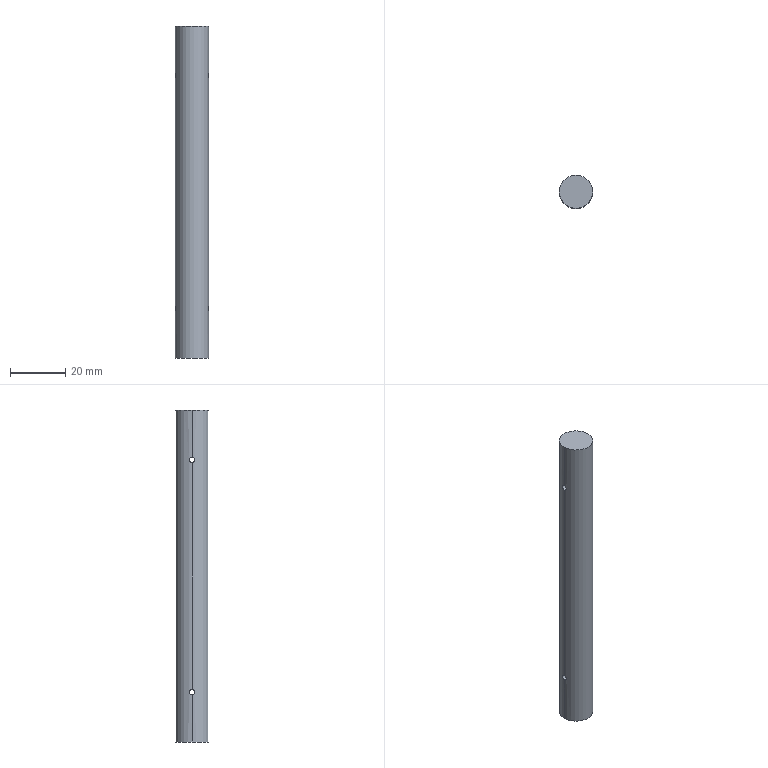Part | SolidWorks | features Cut 1, Extrusion 1 | 1 solid | 8 faces | box 12 x 12 x 120 mm | volume 13497 mm3 | cylinder 6 | plane 2 | commonest cylinder face diameters 2 x4 12 x2
STEP:
#1=CARTESIAN_POINT('',(-94.,71.3,-41.));
#2=VERTEX_POINT('',#1);
#3=CARTESIAN_POINT('',(-94.,71.3,-43.));
#4=VERTEX_POINT('',#3);
#5=CARTESIAN_POINT('',(-94.,71.3,-41.));
#6=CARTESIAN_POINT('',(-94.,71.168,-41.));
#7=CARTESIAN_POINT('',(-94.005,71.038,-41.026));
#8=CARTESIAN_POINT('',(-94.02,70.796,-41.127));
#9=CARTESIAN_POINT('',(-94.031,70.685,-41.201));
#10=CARTESIAN_POINT('',(-94.053,70.501,-41.385));
#11=CARTESIAN_POINT('',(-94.064,70.426,-41.497));
#12=CARTESIAN_POINT('',(-94.079,70.326,-41.737));
#13=CARTESIAN_POINT('',(-94.084,70.3,-41.869));
#14=CARTESIAN_POINT('',(-94.084,70.3,-42.13));
#15=CARTESIAN_POINT('',(-94.079,70.326,-42.261));
#16=CARTESIAN_POINT('',(-94.064,70.426,-42.504));
#17=CARTESIAN_POINT('',(-94.053,70.5,-42.614));
#18=CARTESIAN_POINT('',(-94.031,70.686,-42.8));
#19=CARTESIAN_POINT('',(-94.02,70.796,-42.874));
#20=CARTESIAN_POINT('',(-94.004,71.038,-42.974));
#21=CARTESIAN_POINT('',(-94.,71.169,-43.));
#22=CARTESIAN_POINT('',(-94.,71.3,-43.));
#23=B_SPLINE_CURVE_WITH_KNOTS('',3,(#5,#6,#7,#8,#9,#10,#11,#12,#13,#14,#15,#16,#17,#18,#19,#20,#21,#22),.UNSPECIFIED.,.F.,.F.,(4,2,2,2,2,2,2,2,4),(0.,0.0003915,0.000783,0.001174,0.001566,0.001957,0.002349,0.00274,0.003132),.UNSPECIFIED.);
#24=EDGE_CURVE('',#2,#4,#23,.T.);
#25=ORIENTED_EDGE('',*,*,#24,.T.);
#26=CARTESIAN_POINT('',(-106.,71.3,-43.));
#27=VERTEX_POINT('',#26);
#28=CARTESIAN_POINT('',(-94.,71.3,-43.));
#29=DIRECTION('',(-1.,0.,0.));
#30=VECTOR('',#29,1000.);
#31=LINE('',#28,#30);
#32=EDGE_CURVE('',#4,#27,#31,.T.);
#33=ORIENTED_EDGE('',*,*,#32,.T.);
#34=CARTESIAN_POINT('',(-106.,71.3,-41.));
#35=VERTEX_POINT('',#34);
#36=CARTESIAN_POINT('',(-106.,71.3,-43.));
#37=CARTESIAN_POINT('',(-106.,71.169,-43.));
#38=CARTESIAN_POINT('',(-105.995,71.038,-42.974));
#39=CARTESIAN_POINT('',(-105.98,70.797,-42.874));
#40=CARTESIAN_POINT('',(-105.969,70.686,-42.8));
#41=CARTESIAN_POINT('',(-105.947,70.501,-42.615));
#42=CARTESIAN_POINT('',(-105.936,70.427,-42.505));
#43=CARTESIAN_POINT('',(-105.921,70.326,-42.263));
#44=CARTESIAN_POINT('',(-105.916,70.3,-42.133));
#45=CARTESIAN_POINT('',(-105.916,70.3,-41.868));
#46=CARTESIAN_POINT('',(-105.921,70.326,-41.738));
#47=CARTESIAN_POINT('',(-105.936,70.426,-41.496));
#48=CARTESIAN_POINT('',(-105.947,70.5,-41.385));
#49=CARTESIAN_POINT('',(-105.969,70.684,-41.201));
#50=CARTESIAN_POINT('',(-105.98,70.796,-41.127));
#51=CARTESIAN_POINT('',(-105.995,71.036,-41.027));
#52=CARTESIAN_POINT('',(-106.,71.168,-41.));
#53=CARTESIAN_POINT('',(-106.,71.3,-41.));
#54=B_SPLINE_CURVE_WITH_KNOTS('',3,(#36,#37,#38,#39,#40,#41,#42,#43,#44,#45,#46,#47,#48,#49,#50,#51,#52,#53),.UNSPECIFIED.,.F.,.F.,(4,2,2,2,2,2,2,2,4),(0.003132,0.003523,0.003915,0.004306,0.004697,0.005089,0.00548,0.005872,0.006263),.UNSPECIFIED.);
#55=EDGE_CURVE('',#27,#35,#54,.T.);
#56=ORIENTED_EDGE('',*,*,#55,.T.);
#57=CARTESIAN_POINT('',(-94.,71.3,-41.));
#58=DIRECTION('',(-1.,0.,0.));
#59=VECTOR('',#58,1000.);
#60=LINE('',#57,#59);
#61=EDGE_CURVE('',#2,#35,#60,.T.);
#62=ORIENTED_EDGE('',*,*,#61,.F.);
#63=EDGE_LOOP('',(#25,#33,#56,#62));
#64=FACE_OUTER_BOUND('',#63,.T.);
#65=CARTESIAN_POINT('',(-94.,71.3,-42.));
#66=DIRECTION('',(-1.,0.,0.));
#67=DIRECTION('',(0.,0.,1.));
#68=AXIS2_PLACEMENT_3D('',#65,#66,#67);
#69=CYLINDRICAL_SURFACE('',#68,1.);
#70=ADVANCED_FACE('',(#64),#69,.F.);
#71=CARTESIAN_POINT('',(-94.,71.3,43.));
#72=VERTEX_POINT('',#71);
#73=CARTESIAN_POINT('',(-94.,71.3,41.));
#74=VERTEX_POINT('',#73);
#75=CARTESIAN_POINT('',(-94.,71.3,43.));
#76=CARTESIAN_POINT('',(-94.,71.168,43.));
#77=CARTESIAN_POINT('',(-94.005,71.038,42.974));
#78=CARTESIAN_POINT('',(-94.02,70.796,42.873));
#79=CARTESIAN_POINT('',(-94.031,70.685,42.799));
#80=CARTESIAN_POINT('',(-94.053,70.501,42.615));
#81=CARTESIAN_POINT('',(-94.064,70.426,42.503));
#82=CARTESIAN_POINT('',(-94.079,70.326,42.263));
#83=CARTESIAN_POINT('',(-94.084,70.3,42.131));
#84=CARTESIAN_POINT('',(-94.084,70.3,41.87));
#85=CARTESIAN_POINT('',(-94.079,70.326,41.739));
#86=CARTESIAN_POINT('',(-94.064,70.426,41.496));
#87=CARTESIAN_POINT('',(-94.053,70.5,41.386));
#88=CARTESIAN_POINT('',(-94.031,70.686,41.2));
#89=CARTESIAN_POINT('',(-94.02,70.796,41.126));
#90=CARTESIAN_POINT('',(-94.004,71.038,41.026));
#91=CARTESIAN_POINT('',(-94.,71.169,41.));
#92=CARTESIAN_POINT('',(-94.,71.3,41.));
#93=B_SPLINE_CURVE_WITH_KNOTS('',3,(#75,#76,#77,#78,#79,#80,#81,#82,#83,#84,#85,#86,#87,#88,#89,#90,#91,#92),.UNSPECIFIED.,.F.,.F.,(4,2,2,2,2,2,2,2,4),(0.,0.0003915,0.000783,0.001174,0.001566,0.001957,0.002349,0.00274,0.003132),.UNSPECIFIED.);
#94=EDGE_CURVE('',#72,#74,#93,.T.);
#95=ORIENTED_EDGE('',*,*,#94,.T.);
#96=CARTESIAN_POINT('',(-106.,71.3,41.));
#97=VERTEX_POINT('',#96);
#98=CARTESIAN_POINT('',(-94.,71.3,41.));
#99=DIRECTION('',(-1.,0.,0.));
#100=VECTOR('',#99,1000.);
#101=LINE('',#98,#100);
#102=EDGE_CURVE('',#74,#97,#101,.T.);
#103=ORIENTED_EDGE('',*,*,#102,.T.);
#104=CARTESIAN_POINT('',(-106.,71.3,43.));
#105=VERTEX_POINT('',#104);
#106=CARTESIAN_POINT('',(-106.,71.3,41.));
#107=CARTESIAN_POINT('',(-106.,71.169,41.));
#108=CARTESIAN_POINT('',(-105.995,71.038,41.026));
#109=CARTESIAN_POINT('',(-105.98,70.797,41.126));
#110=CARTESIAN_POINT('',(-105.969,70.686,41.2));
#111=CARTESIAN_POINT('',(-105.947,70.501,41.385));
#112=CARTESIAN_POINT('',(-105.936,70.427,41.495));
#113=CARTESIAN_POINT('',(-105.921,70.326,41.737));
#114=CARTESIAN_POINT('',(-105.916,70.3,41.867));
#115=CARTESIAN_POINT('',(-105.916,70.3,42.132));
#116=CARTESIAN_POINT('',(-105.921,70.326,42.262));
#117=CARTESIAN_POINT('',(-105.936,70.426,42.504));
#118=CARTESIAN_POINT('',(-105.947,70.5,42.615));
#119=CARTESIAN_POINT('',(-105.969,70.684,42.799));
#120=CARTESIAN_POINT('',(-105.98,70.796,42.873));
#121=CARTESIAN_POINT('',(-105.995,71.036,42.973));
#122=CARTESIAN_POINT('',(-106.,71.168,43.));
#123=CARTESIAN_POINT('',(-106.,71.3,43.));
#124=B_SPLINE_CURVE_WITH_KNOTS('',3,(#106,#107,#108,#109,#110,#111,#112,#113,#114,#115,#116,#117,#118,#119,#120,#121,#122,#123),.UNSPECIFIED.,.F.,.F.,(4,2,2,2,2,2,2,2,4),(0.003132,0.003523,0.003915,0.004306,0.004697,0.005089,0.00548,0.005872,0.006263),.UNSPECIFIED.);
#125=EDGE_CURVE('',#97,#105,#124,.T.);
#126=ORIENTED_EDGE('',*,*,#125,.T.);
#127=CARTESIAN_POINT('',(-94.,71.3,43.));
#128=DIRECTION('',(-1.,0.,0.));
#129=VECTOR('',#128,1000.);
#130=LINE('',#127,#129);
#131=EDGE_CURVE('',#72,#105,#130,.T.);
#132=ORIENTED_EDGE('',*,*,#131,.F.);
#133=EDGE_LOOP('',(#95,#103,#126,#132));
#134=FACE_OUTER_BOUND('',#133,.T.);
#135=CARTESIAN_POINT('',(-94.,71.3,42.));
#136=DIRECTION('',(-1.,0.,0.));
#137=DIRECTION('',(0.,0.,1.));
#138=AXIS2_PLACEMENT_3D('',#135,#136,#137);
#139=CYLINDRICAL_SURFACE('',#138,1.);
#140=ADVANCED_FACE('',(#134),#139,.F.);
#141=CARTESIAN_POINT('',(-106.,71.3,-60.));
#142=VERTEX_POINT('',#141);
#143=CARTESIAN_POINT('',(-94.,71.3,-60.));
#144=VERTEX_POINT('',#143);
#145=CARTESIAN_POINT('',(-100.,71.3,-60.));
#146=DIRECTION('',(0.,0.,-1.));
#147=DIRECTION('',(1.,0.,0.));
#148=AXIS2_PLACEMENT_3D('',#145,#146,#147);
#149=CIRCLE('',#148,6.);
#150=EDGE_CURVE('',#142,#144,#149,.T.);
#151=ORIENTED_EDGE('',*,*,#150,.F.);
#152=CARTESIAN_POINT('',(-106.,71.3,-76.971));
#153=DIRECTION('',(0.,0.,1.));
#154=VECTOR('',#153,1000.);
#155=LINE('',#152,#154);
#156=EDGE_CURVE('',#142,#27,#155,.T.);
#157=ORIENTED_EDGE('',*,*,#156,.T.);
#158=CARTESIAN_POINT('',(-106.,71.3,-41.));
#159=CARTESIAN_POINT('',(-106.,71.432,-41.));
#160=CARTESIAN_POINT('',(-105.995,71.562,-41.026));
#161=CARTESIAN_POINT('',(-105.98,71.804,-41.127));
#162=CARTESIAN_POINT('',(-105.969,71.915,-41.201));
#163=CARTESIAN_POINT('',(-105.947,72.099,-41.385));
#164=CARTESIAN_POINT('',(-105.936,72.174,-41.497));
#165=CARTESIAN_POINT('',(-105.921,72.274,-41.737));
#166=CARTESIAN_POINT('',(-105.916,72.3,-41.869));
#167=CARTESIAN_POINT('',(-105.916,72.3,-42.13));
#168=CARTESIAN_POINT('',(-105.921,72.274,-42.261));
#169=CARTESIAN_POINT('',(-105.936,72.174,-42.504));
#170=CARTESIAN_POINT('',(-105.947,72.1,-42.614));
#171=CARTESIAN_POINT('',(-105.969,71.914,-42.8));
#172=CARTESIAN_POINT('',(-105.98,71.804,-42.874));
#173=CARTESIAN_POINT('',(-105.996,71.562,-42.974));
#174=CARTESIAN_POINT('',(-106.,71.431,-43.));
#175=CARTESIAN_POINT('',(-106.,71.3,-43.));
#176=B_SPLINE_CURVE_WITH_KNOTS('',3,(#158,#159,#160,#161,#162,#163,#164,#165,#166,#167,#168,#169,#170,#171,#172,#173,#174,#175),.UNSPECIFIED.,.F.,.F.,(4,2,2,2,2,2,2,2,4),(0.,0.0003915,0.000783,0.001174,0.001566,0.001957,0.002349,0.00274,0.003132),.UNSPECIFIED.);
#177=EDGE_CURVE('',#35,#27,#176,.T.);
#178=ORIENTED_EDGE('',*,*,#177,.F.);
#179=CARTESIAN_POINT('',(-106.,71.3,-76.971));
#180=DIRECTION('',(0.,0.,1.));
#181=VECTOR('',#180,1000.);
#182=LINE('',#179,#181);
#183=EDGE_CURVE('',#35,#97,#182,.T.);
#184=ORIENTED_EDGE('',*,*,#183,.T.);
#185=CARTESIAN_POINT('',(-106.,71.3,43.));
#186=CARTESIAN_POINT('',(-106.,71.432,43.));
#187=CARTESIAN_POINT('',(-105.995,71.562,42.974));
#188=CARTESIAN_POINT('',(-105.98,71.804,42.873));
#189=CARTESIAN_POINT('',(-105.969,71.915,42.799));
#190=CARTESIAN_POINT('',(-105.947,72.099,42.615));
#191=CARTESIAN_POINT('',(-105.936,72.174,42.503));
#192=CARTESIAN_POINT('',(-105.921,72.274,42.263));
#193=CARTESIAN_POINT('',(-105.916,72.3,42.131));
#194=CARTESIAN_POINT('',(-105.916,72.3,41.87));
#195=CARTESIAN_POINT('',(-105.921,72.274,41.739));
#196=CARTESIAN_POINT('',(-105.936,72.174,41.496));
#197=CARTESIAN_POINT('',(-105.947,72.1,41.386));
#198=CARTESIAN_POINT('',(-105.969,71.914,41.2));
#199=CARTESIAN_POINT('',(-105.98,71.804,41.126));
#200=CARTESIAN_POINT('',(-105.996,71.562,41.026));
#201=CARTESIAN_POINT('',(-106.,71.431,41.));
#202=CARTESIAN_POINT('',(-106.,71.3,41.));
#203=B_SPLINE_CURVE_WITH_KNOTS('',3,(#185,#186,#187,#188,#189,#190,#191,#192,#193,#194,#195,#196,#197,#198,#199,#200,#201,#202),.UNSPECIFIED.,.F.,.F.,(4,2,2,2,2,2,2,2,4),(0.,0.0003915,0.000783,0.001174,0.001566,0.001957,0.002349,0.00274,0.003132),.UNSPECIFIED.);
#204=EDGE_CURVE('',#105,#97,#203,.T.);
#205=ORIENTED_EDGE('',*,*,#204,.F.);
#206=CARTESIAN_POINT('',(-106.,71.3,60.));
#207=VERTEX_POINT('',#206);
#208=CARTESIAN_POINT('',(-106.,71.3,-76.971));
#209=DIRECTION('',(0.,0.,1.));
#210=VECTOR('',#209,1000.);
#211=LINE('',#208,#210);
#212=EDGE_CURVE('',#105,#207,#211,.T.);
#213=ORIENTED_EDGE('',*,*,#212,.T.);
#214=CARTESIAN_POINT('',(-94.,71.3,60.));
#215=VERTEX_POINT('',#214);
#216=CARTESIAN_POINT('',(-100.,71.3,60.));
#217=DIRECTION('',(0.,0.,-1.));
#218=DIRECTION('',(-1.,0.,0.));
#219=AXIS2_PLACEMENT_3D('',#216,#217,#218);
#220=CIRCLE('',#219,6.);
#221=EDGE_CURVE('',#207,#215,#220,.T.);
#222=ORIENTED_EDGE('',*,*,#221,.T.);
#223=CARTESIAN_POINT('',(-94.,71.3,-76.971));
#224=DIRECTION('',(0.,0.,1.));
#225=VECTOR('',#224,1000.);
#226=LINE('',#223,#225);
#227=EDGE_CURVE('',#72,#215,#226,.T.);
#228=ORIENTED_EDGE('',*,*,#227,.F.);
#229=CARTESIAN_POINT('',(-94.,71.3,41.));
#230=CARTESIAN_POINT('',(-94.,71.431,41.));
#231=CARTESIAN_POINT('',(-94.005,71.562,41.026));
#232=CARTESIAN_POINT('',(-94.02,71.803,41.126));
#233=CARTESIAN_POINT('',(-94.031,71.914,41.2));
#234=CARTESIAN_POINT('',(-94.053,72.099,41.385));
#235=CARTESIAN_POINT('',(-94.064,72.173,41.495));
#236=CARTESIAN_POINT('',(-94.079,72.274,41.737));
#237=CARTESIAN_POINT('',(-94.084,72.3,41.867));
#238=CARTESIAN_POINT('',(-94.084,72.3,42.132));
#239=CARTESIAN_POINT('',(-94.079,72.274,42.262));
#240=CARTESIAN_POINT('',(-94.064,72.174,42.504));
#241=CARTESIAN_POINT('',(-94.053,72.1,42.615));
#242=CARTESIAN_POINT('',(-94.031,71.916,42.799));
#243=CARTESIAN_POINT('',(-94.02,71.804,42.873));
#244=CARTESIAN_POINT('',(-94.005,71.564,42.973));
#245=CARTESIAN_POINT('',(-94.,71.432,43.));
#246=CARTESIAN_POINT('',(-94.,71.3,43.));
#247=B_SPLINE_CURVE_WITH_KNOTS('',3,(#229,#230,#231,#232,#233,#234,#235,#236,#237,#238,#239,#240,#241,#242,#243,#244,#245,#246),.UNSPECIFIED.,.F.,.F.,(4,2,2,2,2,2,2,2,4),(0.003132,0.003523,0.003915,0.004306,0.004697,0.005089,0.00548,0.005872,0.006263),.UNSPECIFIED.);
#248=EDGE_CURVE('',#74,#72,#247,.T.);
#249=ORIENTED_EDGE('',*,*,#248,.F.);
#250=CARTESIAN_POINT('',(-94.,71.3,-76.971));
#251=DIRECTION('',(0.,0.,1.));
#252=VECTOR('',#251,1000.);
#253=LINE('',#250,#252);
#254=EDGE_CURVE('',#2,#74,#253,.T.);
#255=ORIENTED_EDGE('',*,*,#254,.F.);
#256=CARTESIAN_POINT('',(-94.,71.3,-43.));
#257=CARTESIAN_POINT('',(-94.,71.431,-43.));
#258=CARTESIAN_POINT('',(-94.005,71.562,-42.974));
#259=CARTESIAN_POINT('',(-94.02,71.803,-42.874));
#260=CARTESIAN_POINT('',(-94.031,71.914,-42.8));
#261=CARTESIAN_POINT('',(-94.053,72.099,-42.615));
#262=CARTESIAN_POINT('',(-94.064,72.173,-42.505));
#263=CARTESIAN_POINT('',(-94.079,72.274,-42.263));
#264=CARTESIAN_POINT('',(-94.084,72.3,-42.133));
#265=CARTESIAN_POINT('',(-94.084,72.3,-41.868));
#266=CARTESIAN_POINT('',(-94.079,72.274,-41.738));
#267=CARTESIAN_POINT('',(-94.064,72.174,-41.496));
#268=CARTESIAN_POINT('',(-94.053,72.1,-41.385));
#269=CARTESIAN_POINT('',(-94.031,71.916,-41.201));
#270=CARTESIAN_POINT('',(-94.02,71.804,-41.127));
#271=CARTESIAN_POINT('',(-94.005,71.564,-41.027));
#272=CARTESIAN_POINT('',(-94.,71.432,-41.));
#273=CARTESIAN_POINT('',(-94.,71.3,-41.));
#274=B_SPLINE_CURVE_WITH_KNOTS('',3,(#256,#257,#258,#259,#260,#261,#262,#263,#264,#265,#266,#267,#268,#269,#270,#271,#272,#273),.UNSPECIFIED.,.F.,.F.,(4,2,2,2,2,2,2,2,4),(0.003132,0.003523,0.003915,0.004306,0.004697,0.005089,0.00548,0.005872,0.006263),.UNSPECIFIED.);
#275=EDGE_CURVE('',#4,#2,#274,.T.);
#276=ORIENTED_EDGE('',*,*,#275,.F.);
#277=CARTESIAN_POINT('',(-94.,71.3,-76.971));
#278=DIRECTION('',(0.,0.,1.));
#279=VECTOR('',#278,1000.);
#280=LINE('',#277,#279);
#281=EDGE_CURVE('',#144,#4,#280,.T.);
#282=ORIENTED_EDGE('',*,*,#281,.F.);
#283=EDGE_LOOP('',(#151,#157,#178,#184,#205,#213,#222,#228,#249,#255,#276,#282));
#284=FACE_OUTER_BOUND('',#283,.T.);
#285=CARTESIAN_POINT('',(-100.,71.3,-76.971));
#286=DIRECTION('',(0.,0.,1.));
#287=DIRECTION('',(1.,0.,0.));
#288=AXIS2_PLACEMENT_3D('',#285,#286,#287);
#289=CYLINDRICAL_SURFACE('',#288,6.);
#290=ADVANCED_FACE('',(#284),#289,.T.);
#291=ORIENTED_EDGE('',*,*,#156,.F.);
#292=CARTESIAN_POINT('',(-100.,71.3,-60.));
#293=DIRECTION('',(0.,0.,-1.));
#294=DIRECTION('',(1.,0.,0.));
#295=AXIS2_PLACEMENT_3D('',#292,#293,#294);
#296=CIRCLE('',#295,6.);
#297=EDGE_CURVE('',#144,#142,#296,.T.);
#298=ORIENTED_EDGE('',*,*,#297,.F.);
#299=ORIENTED_EDGE('',*,*,#281,.T.);
#300=ORIENTED_EDGE('',*,*,#24,.F.);
#301=ORIENTED_EDGE('',*,*,#254,.T.);
#302=ORIENTED_EDGE('',*,*,#94,.F.);
#303=ORIENTED_EDGE('',*,*,#227,.T.);
#304=CARTESIAN_POINT('',(-100.,71.3,60.));
#305=DIRECTION('',(0.,0.,-1.));
#306=DIRECTION('',(-1.,0.,0.));
#307=AXIS2_PLACEMENT_3D('',#304,#305,#306);
#308=CIRCLE('',#307,6.);
#309=EDGE_CURVE('',#215,#207,#308,.T.);
#310=ORIENTED_EDGE('',*,*,#309,.T.);
#311=ORIENTED_EDGE('',*,*,#212,.F.);
#312=ORIENTED_EDGE('',*,*,#125,.F.);
#313=ORIENTED_EDGE('',*,*,#183,.F.);
#314=ORIENTED_EDGE('',*,*,#55,.F.);
#315=EDGE_LOOP('',(#291,#298,#299,#300,#301,#302,#303,#310,#311,#312,#313,#314));
#316=FACE_OUTER_BOUND('',#315,.T.);
#317=CARTESIAN_POINT('',(-100.,71.3,-76.971));
#318=DIRECTION('',(0.,0.,1.));
#319=DIRECTION('',(1.,0.,0.));
#320=AXIS2_PLACEMENT_3D('',#317,#318,#319);
#321=CYLINDRICAL_SURFACE('',#320,6.);
#322=ADVANCED_FACE('',(#316),#321,.T.);
#323=ORIENTED_EDGE('',*,*,#297,.T.);
#324=ORIENTED_EDGE('',*,*,#150,.T.);
#325=EDGE_LOOP('',(#323,#324));
#326=FACE_OUTER_BOUND('',#325,.T.);
#327=CARTESIAN_POINT('',(-70.,-20.,-60.));
#328=DIRECTION('',(0.,0.,1.));
#329=DIRECTION('',(-1.,0.,0.));
#330=AXIS2_PLACEMENT_3D('',#327,#328,#329);
#331=PLANE('',#330);
#332=ADVANCED_FACE('',(#326),#331,.F.);
#333=ORIENTED_EDGE('',*,*,#309,.F.);
#334=ORIENTED_EDGE('',*,*,#221,.F.);
#335=EDGE_LOOP('',(#333,#334));
#336=FACE_OUTER_BOUND('',#335,.T.);
#337=CARTESIAN_POINT('',(-70.,-20.,60.));
#338=DIRECTION('',(0.,0.,-1.));
#339=DIRECTION('',(1.,0.,0.));
#340=AXIS2_PLACEMENT_3D('',#337,#338,#339);
#341=PLANE('',#340);
#342=ADVANCED_FACE('',(#336),#341,.F.);
#343=ORIENTED_EDGE('',*,*,#102,.F.);
#344=ORIENTED_EDGE('',*,*,#248,.T.);
#345=ORIENTED_EDGE('',*,*,#131,.T.);
#346=ORIENTED_EDGE('',*,*,#204,.T.);
#347=EDGE_LOOP('',(#343,#344,#345,#346));
#348=FACE_OUTER_BOUND('',#347,.T.);
#349=CARTESIAN_POINT('',(-94.,71.3,42.));
#350=DIRECTION('',(-1.,0.,0.));
#351=DIRECTION('',(0.,0.,1.));
#352=AXIS2_PLACEMENT_3D('',#349,#350,#351);
#353=CYLINDRICAL_SURFACE('',#352,1.);
#354=ADVANCED_FACE('',(#348),#353,.F.);
#355=ORIENTED_EDGE('',*,*,#32,.F.);
#356=ORIENTED_EDGE('',*,*,#275,.T.);
#357=ORIENTED_EDGE('',*,*,#61,.T.);
#358=ORIENTED_EDGE('',*,*,#177,.T.);
#359=EDGE_LOOP('',(#355,#356,#357,#358));
#360=FACE_OUTER_BOUND('',#359,.T.);
#361=CARTESIAN_POINT('',(-94.,71.3,-42.));
#362=DIRECTION('',(-1.,0.,0.));
#363=DIRECTION('',(0.,0.,1.));
#364=AXIS2_PLACEMENT_3D('',#361,#362,#363);
#365=CYLINDRICAL_SURFACE('',#364,1.);
#366=ADVANCED_FACE('',(#360),#365,.F.);
#367=CLOSED_SHELL('',(#70,#140,#290,#322,#332,#342,#354,#366));
#368=MANIFOLD_SOLID_BREP('',#367);
#369=CARTESIAN_POINT('',(0.,0.,0.));
#370=DIRECTION('',(0.,0.,1.));
#371=DIRECTION('',(1.,0.,0.));
#372=AXIS2_PLACEMENT_3D('',#369,#370,#371);
#373=(LENGTH_UNIT()NAMED_UNIT(*)SI_UNIT(.MILLI.,.METRE.));
#374=UNCERTAINTY_MEASURE_WITH_UNIT(LENGTH_MEASURE(0.00001),#373,'','');
#375=(NAMED_UNIT(*)PLANE_ANGLE_UNIT()SI_UNIT($,.RADIAN.));
#376=(NAMED_UNIT(*)SI_UNIT($,.STERADIAN.)SOLID_ANGLE_UNIT());
#377=(GEOMETRIC_REPRESENTATION_CONTEXT(3)GLOBAL_UNCERTAINTY_ASSIGNED_CONTEXT((#374))GLOBAL_UNIT_ASSIGNED_CONTEXT((#373,#375,#376))REPRESENTATION_CONTEXT('',''));
#378=ADVANCED_BREP_SHAPE_REPRESENTATION('',(#368,#372),#377);